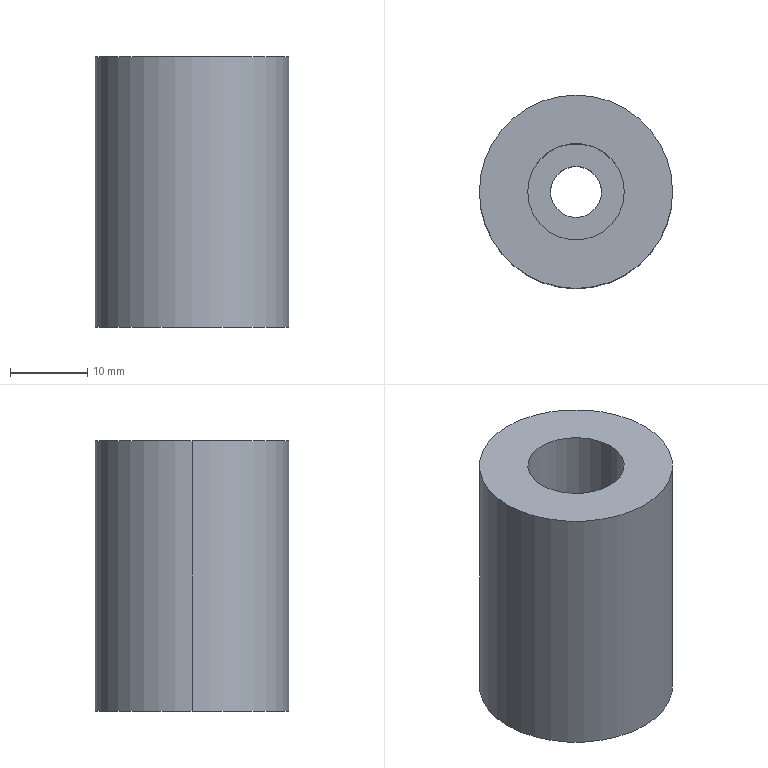Part | SolidWorks | features BaseBody 1 | 1 solid | 9 faces | box 25 x 25 x 35 mm | volume 14656 mm3 | cylinder 6 | plane 3 | commonest cylinder face diameters 6.6 x2 12.5 x2 25 x2
STEP:
#1=CARTESIAN_POINT('',(-12.5,0.,35.));
#2=VERTEX_POINT('',#1);
#3=CARTESIAN_POINT('',(12.5,0.,35.));
#4=VERTEX_POINT('',#3);
#5=CARTESIAN_POINT('',(0.,0.,35.));
#6=DIRECTION('',(0.,0.,-1.));
#7=DIRECTION('',(-1.,0.,0.));
#8=AXIS2_PLACEMENT_3D('',#5,#6,#7);
#9=CIRCLE('',#8,12.5);
#10=EDGE_CURVE('',#2,#4,#9,.T.);
#11=ORIENTED_EDGE('',*,*,#10,.T.);
#12=CARTESIAN_POINT('',(12.5,0.,0.));
#13=VERTEX_POINT('',#12);
#14=CARTESIAN_POINT('',(12.5,0.,35.));
#15=DIRECTION('',(0.,0.,-1.));
#16=VECTOR('',#15,1000.);
#17=LINE('',#14,#16);
#18=EDGE_CURVE('',#4,#13,#17,.T.);
#19=ORIENTED_EDGE('',*,*,#18,.T.);
#20=CARTESIAN_POINT('',(-12.5,0.,0.));
#21=VERTEX_POINT('',#20);
#22=CARTESIAN_POINT('',(0.,0.,0.));
#23=DIRECTION('',(0.,0.,1.));
#24=DIRECTION('',(-1.,0.,0.));
#25=AXIS2_PLACEMENT_3D('',#22,#23,#24);
#26=CIRCLE('',#25,12.5);
#27=EDGE_CURVE('',#13,#21,#26,.T.);
#28=ORIENTED_EDGE('',*,*,#27,.T.);
#29=CARTESIAN_POINT('',(-12.5,0.,35.));
#30=DIRECTION('',(0.,0.,-1.));
#31=VECTOR('',#30,1000.);
#32=LINE('',#29,#31);
#33=EDGE_CURVE('',#2,#21,#32,.T.);
#34=ORIENTED_EDGE('',*,*,#33,.F.);
#35=EDGE_LOOP('',(#11,#19,#28,#34));
#36=FACE_OUTER_BOUND('',#35,.T.);
#37=CARTESIAN_POINT('',(0.,0.,35.));
#38=DIRECTION('',(0.,0.,-1.));
#39=DIRECTION('',(-1.,0.,0.));
#40=AXIS2_PLACEMENT_3D('',#37,#38,#39);
#41=CYLINDRICAL_SURFACE('',#40,12.5);
#42=ADVANCED_FACE('',(#36),#41,.T.);
#43=CARTESIAN_POINT('',(3.3,0.,0.));
#44=VERTEX_POINT('',#43);
#45=CARTESIAN_POINT('',(-3.3,0.,0.));
#46=VERTEX_POINT('',#45);
#47=CARTESIAN_POINT('',(0.,0.,0.));
#48=DIRECTION('',(0.,0.,-1.));
#49=DIRECTION('',(1.,0.,0.));
#50=AXIS2_PLACEMENT_3D('',#47,#48,#49);
#51=CIRCLE('',#50,3.3);
#52=EDGE_CURVE('',#44,#46,#51,.T.);
#53=ORIENTED_EDGE('',*,*,#52,.T.);
#54=CARTESIAN_POINT('',(-3.3,0.,20.));
#55=VERTEX_POINT('',#54);
#56=CARTESIAN_POINT('',(-3.3,0.,35.));
#57=DIRECTION('',(0.,0.,1.));
#58=VECTOR('',#57,1000.);
#59=LINE('',#56,#58);
#60=EDGE_CURVE('',#46,#55,#59,.T.);
#61=ORIENTED_EDGE('',*,*,#60,.T.);
#62=CARTESIAN_POINT('',(3.3,0.,20.));
#63=VERTEX_POINT('',#62);
#64=CARTESIAN_POINT('',(0.,0.,20.));
#65=DIRECTION('',(0.,0.,-1.));
#66=DIRECTION('',(1.,0.,0.));
#67=AXIS2_PLACEMENT_3D('',#64,#65,#66);
#68=CIRCLE('',#67,3.3);
#69=EDGE_CURVE('',#63,#55,#68,.T.);
#70=ORIENTED_EDGE('',*,*,#69,.F.);
#71=CARTESIAN_POINT('',(3.3,0.,35.));
#72=DIRECTION('',(0.,0.,1.));
#73=VECTOR('',#72,1000.);
#74=LINE('',#71,#73);
#75=EDGE_CURVE('',#44,#63,#74,.T.);
#76=ORIENTED_EDGE('',*,*,#75,.F.);
#77=EDGE_LOOP('',(#53,#61,#70,#76));
#78=FACE_OUTER_BOUND('',#77,.T.);
#79=CARTESIAN_POINT('',(0.,0.,35.));
#80=DIRECTION('',(0.,0.,1.));
#81=DIRECTION('',(1.,0.,0.));
#82=AXIS2_PLACEMENT_3D('',#79,#80,#81);
#83=CYLINDRICAL_SURFACE('',#82,3.3);
#84=ADVANCED_FACE('',(#78),#83,.F.);
#85=CARTESIAN_POINT('',(-6.25,0.,20.));
#86=VERTEX_POINT('',#85);
#87=CARTESIAN_POINT('',(6.25,0.,20.));
#88=VERTEX_POINT('',#87);
#89=CARTESIAN_POINT('',(0.,0.,20.));
#90=DIRECTION('',(0.,0.,1.));
#91=DIRECTION('',(1.,0.,0.));
#92=AXIS2_PLACEMENT_3D('',#89,#90,#91);
#93=CIRCLE('',#92,6.25);
#94=EDGE_CURVE('',#86,#88,#93,.T.);
#95=ORIENTED_EDGE('',*,*,#94,.F.);
#96=CARTESIAN_POINT('',(-6.25,0.,35.));
#97=VERTEX_POINT('',#96);
#98=CARTESIAN_POINT('',(-6.25,0.,35.));
#99=DIRECTION('',(0.,0.,1.));
#100=VECTOR('',#99,1000.);
#101=LINE('',#98,#100);
#102=EDGE_CURVE('',#86,#97,#101,.T.);
#103=ORIENTED_EDGE('',*,*,#102,.T.);
#104=CARTESIAN_POINT('',(6.25,0.,35.));
#105=VERTEX_POINT('',#104);
#106=CARTESIAN_POINT('',(0.,0.,35.));
#107=DIRECTION('',(0.,0.,-1.));
#108=DIRECTION('',(1.,0.,0.));
#109=AXIS2_PLACEMENT_3D('',#106,#107,#108);
#110=CIRCLE('',#109,6.25);
#111=EDGE_CURVE('',#105,#97,#110,.T.);
#112=ORIENTED_EDGE('',*,*,#111,.F.);
#113=CARTESIAN_POINT('',(6.25,0.,35.));
#114=DIRECTION('',(0.,0.,1.));
#115=VECTOR('',#114,1000.);
#116=LINE('',#113,#115);
#117=EDGE_CURVE('',#88,#105,#116,.T.);
#118=ORIENTED_EDGE('',*,*,#117,.F.);
#119=EDGE_LOOP('',(#95,#103,#112,#118));
#120=FACE_OUTER_BOUND('',#119,.T.);
#121=CARTESIAN_POINT('',(0.,0.,35.));
#122=DIRECTION('',(0.,0.,1.));
#123=DIRECTION('',(1.,0.,0.));
#124=AXIS2_PLACEMENT_3D('',#121,#122,#123);
#125=CYLINDRICAL_SURFACE('',#124,6.25);
#126=ADVANCED_FACE('',(#120),#125,.F.);
#127=ORIENTED_EDGE('',*,*,#18,.F.);
#128=CARTESIAN_POINT('',(0.,0.,35.));
#129=DIRECTION('',(0.,0.,-1.));
#130=DIRECTION('',(-1.,0.,0.));
#131=AXIS2_PLACEMENT_3D('',#128,#129,#130);
#132=CIRCLE('',#131,12.5);
#133=EDGE_CURVE('',#4,#2,#132,.T.);
#134=ORIENTED_EDGE('',*,*,#133,.T.);
#135=ORIENTED_EDGE('',*,*,#33,.T.);
#136=CARTESIAN_POINT('',(0.,0.,0.));
#137=DIRECTION('',(0.,0.,1.));
#138=DIRECTION('',(-1.,0.,0.));
#139=AXIS2_PLACEMENT_3D('',#136,#137,#138);
#140=CIRCLE('',#139,12.5);
#141=EDGE_CURVE('',#21,#13,#140,.T.);
#142=ORIENTED_EDGE('',*,*,#141,.T.);
#143=EDGE_LOOP('',(#127,#134,#135,#142));
#144=FACE_OUTER_BOUND('',#143,.T.);
#145=CARTESIAN_POINT('',(0.,0.,35.));
#146=DIRECTION('',(0.,0.,-1.));
#147=DIRECTION('',(-1.,0.,0.));
#148=AXIS2_PLACEMENT_3D('',#145,#146,#147);
#149=CYLINDRICAL_SURFACE('',#148,12.5);
#150=ADVANCED_FACE('',(#144),#149,.T.);
#151=ORIENTED_EDGE('',*,*,#141,.F.);
#152=ORIENTED_EDGE('',*,*,#27,.F.);
#153=EDGE_LOOP('',(#151,#152));
#154=FACE_OUTER_BOUND('',#153,.T.);
#155=ORIENTED_EDGE('',*,*,#52,.F.);
#156=CARTESIAN_POINT('',(0.,0.,0.));
#157=DIRECTION('',(0.,0.,-1.));
#158=DIRECTION('',(1.,0.,0.));
#159=AXIS2_PLACEMENT_3D('',#156,#157,#158);
#160=CIRCLE('',#159,3.3);
#161=EDGE_CURVE('',#46,#44,#160,.T.);
#162=ORIENTED_EDGE('',*,*,#161,.F.);
#163=EDGE_LOOP('',(#155,#162));
#164=FACE_BOUND('',#163,.T.);
#165=CARTESIAN_POINT('',(0.,0.,0.));
#166=DIRECTION('',(0.,0.,1.));
#167=DIRECTION('',(1.,0.,0.));
#168=AXIS2_PLACEMENT_3D('',#165,#166,#167);
#169=PLANE('',#168);
#170=ADVANCED_FACE('',(#154,#164),#169,.F.);
#171=ORIENTED_EDGE('',*,*,#10,.F.);
#172=ORIENTED_EDGE('',*,*,#133,.F.);
#173=EDGE_LOOP('',(#171,#172));
#174=FACE_OUTER_BOUND('',#173,.T.);
#175=ORIENTED_EDGE('',*,*,#111,.T.);
#176=CARTESIAN_POINT('',(0.,0.,35.));
#177=DIRECTION('',(0.,0.,-1.));
#178=DIRECTION('',(1.,0.,0.));
#179=AXIS2_PLACEMENT_3D('',#176,#177,#178);
#180=CIRCLE('',#179,6.25);
#181=EDGE_CURVE('',#97,#105,#180,.T.);
#182=ORIENTED_EDGE('',*,*,#181,.T.);
#183=EDGE_LOOP('',(#175,#182));
#184=FACE_BOUND('',#183,.T.);
#185=CARTESIAN_POINT('',(0.,0.,35.));
#186=DIRECTION('',(0.,0.,1.));
#187=DIRECTION('',(1.,0.,0.));
#188=AXIS2_PLACEMENT_3D('',#185,#186,#187);
#189=PLANE('',#188);
#190=ADVANCED_FACE('',(#174,#184),#189,.T.);
#191=ORIENTED_EDGE('',*,*,#60,.F.);
#192=ORIENTED_EDGE('',*,*,#161,.T.);
#193=ORIENTED_EDGE('',*,*,#75,.T.);
#194=CARTESIAN_POINT('',(0.,0.,20.));
#195=DIRECTION('',(0.,0.,-1.));
#196=DIRECTION('',(1.,0.,0.));
#197=AXIS2_PLACEMENT_3D('',#194,#195,#196);
#198=CIRCLE('',#197,3.3);
#199=EDGE_CURVE('',#55,#63,#198,.T.);
#200=ORIENTED_EDGE('',*,*,#199,.F.);
#201=EDGE_LOOP('',(#191,#192,#193,#200));
#202=FACE_OUTER_BOUND('',#201,.T.);
#203=CARTESIAN_POINT('',(0.,0.,35.));
#204=DIRECTION('',(0.,0.,1.));
#205=DIRECTION('',(1.,0.,0.));
#206=AXIS2_PLACEMENT_3D('',#203,#204,#205);
#207=CYLINDRICAL_SURFACE('',#206,3.3);
#208=ADVANCED_FACE('',(#202),#207,.F.);
#209=ORIENTED_EDGE('',*,*,#102,.F.);
#210=CARTESIAN_POINT('',(0.,0.,20.));
#211=DIRECTION('',(0.,0.,1.));
#212=DIRECTION('',(1.,0.,0.));
#213=AXIS2_PLACEMENT_3D('',#210,#211,#212);
#214=CIRCLE('',#213,6.25);
#215=EDGE_CURVE('',#88,#86,#214,.T.);
#216=ORIENTED_EDGE('',*,*,#215,.F.);
#217=ORIENTED_EDGE('',*,*,#117,.T.);
#218=ORIENTED_EDGE('',*,*,#181,.F.);
#219=EDGE_LOOP('',(#209,#216,#217,#218));
#220=FACE_OUTER_BOUND('',#219,.T.);
#221=CARTESIAN_POINT('',(0.,0.,35.));
#222=DIRECTION('',(0.,0.,1.));
#223=DIRECTION('',(1.,0.,0.));
#224=AXIS2_PLACEMENT_3D('',#221,#222,#223);
#225=CYLINDRICAL_SURFACE('',#224,6.25);
#226=ADVANCED_FACE('',(#220),#225,.F.);
#227=ORIENTED_EDGE('',*,*,#215,.T.);
#228=ORIENTED_EDGE('',*,*,#94,.T.);
#229=EDGE_LOOP('',(#227,#228));
#230=FACE_OUTER_BOUND('',#229,.T.);
#231=ORIENTED_EDGE('',*,*,#69,.T.);
#232=ORIENTED_EDGE('',*,*,#199,.T.);
#233=EDGE_LOOP('',(#231,#232));
#234=FACE_BOUND('',#233,.T.);
#235=CARTESIAN_POINT('',(3.3,0.,20.));
#236=DIRECTION('',(0.,0.,-1.));
#237=DIRECTION('',(-1.,0.,0.));
#238=AXIS2_PLACEMENT_3D('',#235,#236,#237);
#239=PLANE('',#238);
#240=ADVANCED_FACE('',(#230,#234),#239,.F.);
#241=CLOSED_SHELL('',(#42,#84,#126,#150,#170,#190,#208,#226,#240));
#242=MANIFOLD_SOLID_BREP('',#241);
#243=CARTESIAN_POINT('',(0.,0.,0.));
#244=DIRECTION('',(0.,0.,1.));
#245=DIRECTION('',(1.,0.,0.));
#246=AXIS2_PLACEMENT_3D('',#243,#244,#245);
#247=(LENGTH_UNIT()NAMED_UNIT(*)SI_UNIT(.MILLI.,.METRE.));
#248=UNCERTAINTY_MEASURE_WITH_UNIT(LENGTH_MEASURE(0.00001),#247,'','');
#249=(NAMED_UNIT(*)PLANE_ANGLE_UNIT()SI_UNIT($,.RADIAN.));
#250=(NAMED_UNIT(*)SI_UNIT($,.STERADIAN.)SOLID_ANGLE_UNIT());
#251=(GEOMETRIC_REPRESENTATION_CONTEXT(3)GLOBAL_UNCERTAINTY_ASSIGNED_CONTEXT((#248))GLOBAL_UNIT_ASSIGNED_CONTEXT((#247,#249,#250))REPRESENTATION_CONTEXT('',''));
#252=ADVANCED_BREP_SHAPE_REPRESENTATION('',(#242,#246),#251);